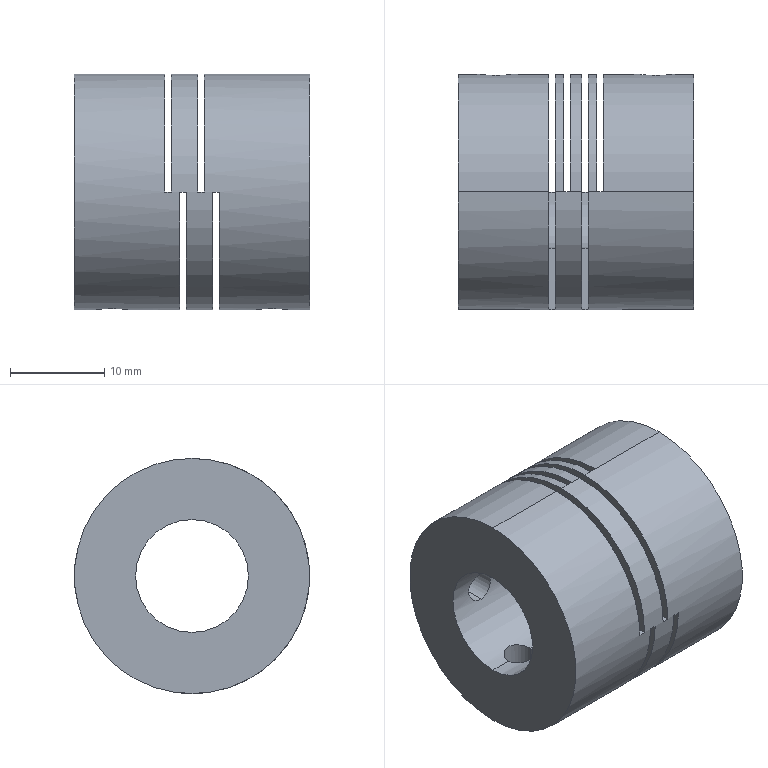Part | STEP file | Coupling CPSφ12-φ12-φ25 | 1 solid | 38 faces | box 25 x 25 x 25 mm | volume 8428 mm3 | cylinder 20 | plane 18 | commonest cylinder face diameters 3.3 x8 12 x6 25 x6